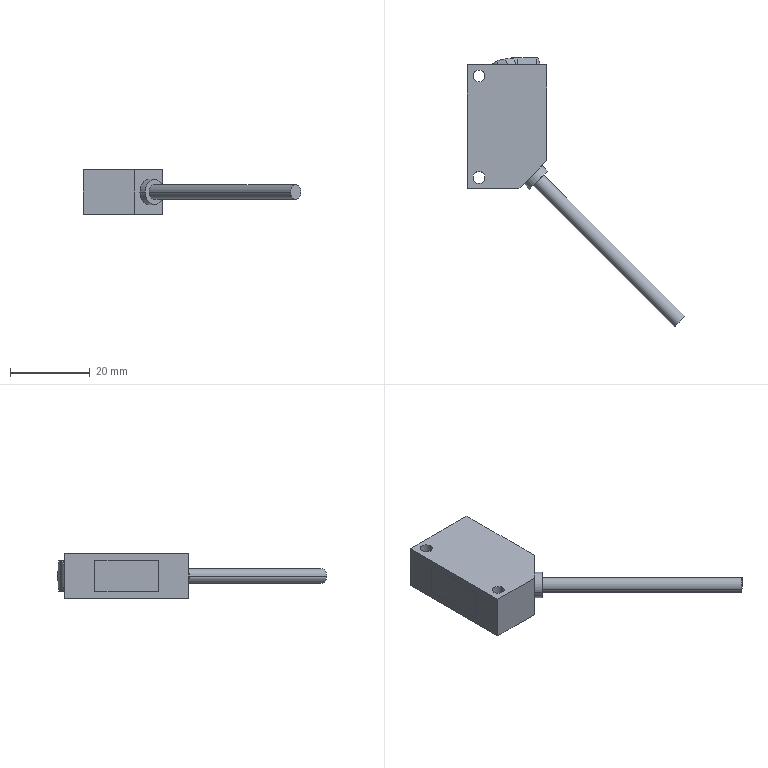Part | SolidWorks | features BaseBody 1 | 1 solid | 60 faces | box 54.507 x 67.407 x 11.2 mm | volume 7195 mm3 | plane 30 | cylinder 24 | cone 4 | spline 2 | commonest cylinder face diameters 2.2 x10 3 x4 2 x2 3.6 x2 3.7 x2 6.4 x2